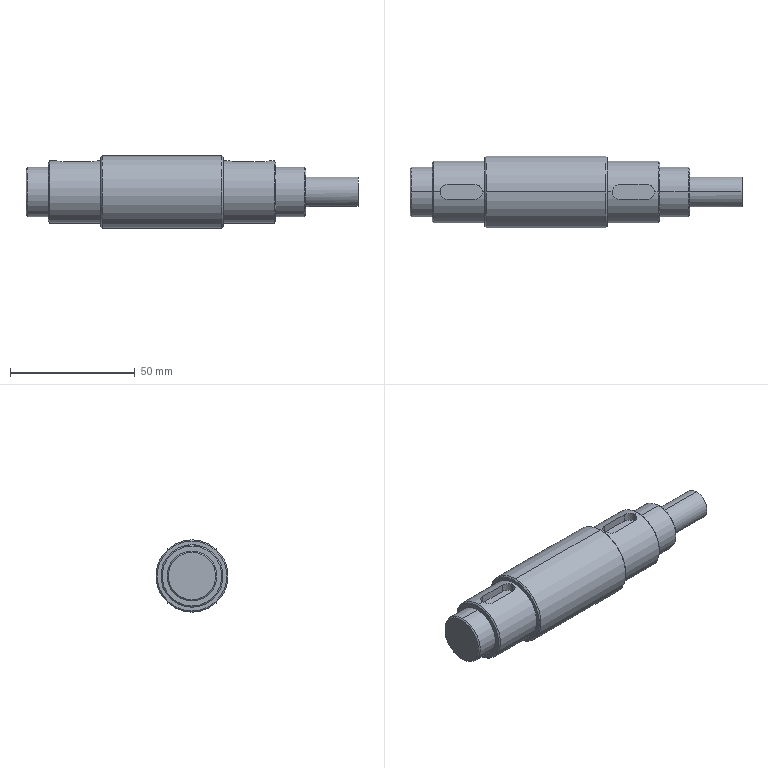Part | NX | features BREP 1 | 1 solid | 52 faces | box 133 x 29 x 29 mm | volume 61010 mm3 | cylinder 22 | plane 16 | cone 14 | commonest cylinder face diameters 6 x6 20 x4 25 x4 3.3 x2 4 x2 12 x2
STEP:
#1=CARTESIAN_POINT('',(-45.5,0.,12.));
#2=VERTEX_POINT('',#1);
#3=CARTESIAN_POINT('',(-45.5,0.,-12.));
#4=VERTEX_POINT('',#3);
#5=CARTESIAN_POINT('',(-45.5,0.,0.));
#6=DIRECTION('',(-1.,0.,0.));
#7=DIRECTION('',(0.,0.,-1.));
#8=AXIS2_PLACEMENT_3D('',#5,#6,#7);
#9=CIRCLE('',#8,12.);
#10=EDGE_CURVE('',#2,#4,#9,.T.);
#11=ORIENTED_EDGE('',*,*,#10,.F.);
#12=CARTESIAN_POINT('',(-45.,0.,12.5));
#13=VERTEX_POINT('',#12);
#14=CARTESIAN_POINT('',(-45.5,0.,12.));
#15=DIRECTION('',(0.7071,0.,0.7071));
#16=VECTOR('',#15,1000.);
#17=LINE('',#14,#16);
#18=EDGE_CURVE('',#2,#13,#17,.T.);
#19=ORIENTED_EDGE('',*,*,#18,.T.);
#20=CARTESIAN_POINT('',(-45.,0.,-12.5));
#21=VERTEX_POINT('',#20);
#22=CARTESIAN_POINT('',(-45.,0.,0.));
#23=DIRECTION('',(1.,0.,0.));
#24=DIRECTION('',(0.,0.,-1.));
#25=AXIS2_PLACEMENT_3D('',#22,#23,#24);
#26=CIRCLE('',#25,12.5);
#27=EDGE_CURVE('',#21,#13,#26,.T.);
#28=ORIENTED_EDGE('',*,*,#27,.F.);
#29=CARTESIAN_POINT('',(-45.5,0.,-12.));
#30=DIRECTION('',(0.7071,0.,-0.7071));
#31=VECTOR('',#30,1000.);
#32=LINE('',#29,#31);
#33=EDGE_CURVE('',#4,#21,#32,.T.);
#34=ORIENTED_EDGE('',*,*,#33,.F.);
#35=EDGE_LOOP('',(#11,#19,#28,#34));
#36=FACE_BOUND('',#35,.T.);
#37=CARTESIAN_POINT('',(-45.5,0.,0.));
#38=DIRECTION('',(1.,0.,0.));
#39=DIRECTION('',(0.,0.,-1.));
#40=AXIS2_PLACEMENT_3D('',#37,#38,#39);
#41=CONICAL_SURFACE('',#40,12.,0.7854);
#42=ADVANCED_FACE('',(#36),#41,.T.);
#43=CARTESIAN_POINT('',(45.5,0.,-12.));
#44=VERTEX_POINT('',#43);
#45=CARTESIAN_POINT('',(45.5,0.,12.));
#46=VERTEX_POINT('',#45);
#47=CARTESIAN_POINT('',(45.5,0.,0.));
#48=DIRECTION('',(1.,0.,0.));
#49=DIRECTION('',(0.,0.,1.));
#50=AXIS2_PLACEMENT_3D('',#47,#48,#49);
#51=CIRCLE('',#50,12.);
#52=EDGE_CURVE('',#44,#46,#51,.T.);
#53=ORIENTED_EDGE('',*,*,#52,.F.);
#54=CARTESIAN_POINT('',(45.,0.,-12.5));
#55=VERTEX_POINT('',#54);
#56=CARTESIAN_POINT('',(45.,0.,-12.5));
#57=DIRECTION('',(-0.7071,0.,-0.7071));
#58=VECTOR('',#57,1000.);
#59=LINE('',#56,#58);
#60=EDGE_CURVE('',#55,#44,#59,.F.);
#61=ORIENTED_EDGE('',*,*,#60,.F.);
#62=CARTESIAN_POINT('',(45.,0.,12.5));
#63=VERTEX_POINT('',#62);
#64=CARTESIAN_POINT('',(45.,0.,0.));
#65=DIRECTION('',(-1.,0.,0.));
#66=DIRECTION('',(0.,0.,1.));
#67=AXIS2_PLACEMENT_3D('',#64,#65,#66);
#68=CIRCLE('',#67,12.5);
#69=EDGE_CURVE('',#63,#55,#68,.T.);
#70=ORIENTED_EDGE('',*,*,#69,.F.);
#71=CARTESIAN_POINT('',(45.,0.,12.5));
#72=DIRECTION('',(-0.7071,0.,0.7071));
#73=VECTOR('',#72,1000.);
#74=LINE('',#71,#73);
#75=EDGE_CURVE('',#63,#46,#74,.F.);
#76=ORIENTED_EDGE('',*,*,#75,.T.);
#77=EDGE_LOOP('',(#53,#61,#70,#76));
#78=FACE_BOUND('',#77,.T.);
#79=CARTESIAN_POINT('',(45.,0.,0.));
#80=DIRECTION('',(-1.,0.,0.));
#81=DIRECTION('',(0.,0.,1.));
#82=AXIS2_PLACEMENT_3D('',#79,#80,#81);
#83=CONICAL_SURFACE('',#82,12.5,0.7854);
#84=ADVANCED_FACE('',(#78),#83,.T.);
#85=CARTESIAN_POINT('',(-24.5,0.,14.));
#86=VERTEX_POINT('',#85);
#87=CARTESIAN_POINT('',(-24.5,0.,-14.));
#88=VERTEX_POINT('',#87);
#89=CARTESIAN_POINT('',(-24.5,0.,0.));
#90=DIRECTION('',(-1.,0.,0.));
#91=DIRECTION('',(0.,0.,-1.));
#92=AXIS2_PLACEMENT_3D('',#89,#90,#91);
#93=CIRCLE('',#92,14.);
#94=EDGE_CURVE('',#86,#88,#93,.T.);
#95=ORIENTED_EDGE('',*,*,#94,.F.);
#96=CARTESIAN_POINT('',(-24.,0.,14.5));
#97=VERTEX_POINT('',#96);
#98=CARTESIAN_POINT('',(-24.5,0.,14.));
#99=DIRECTION('',(0.7071,0.,0.7071));
#100=VECTOR('',#99,1000.);
#101=LINE('',#98,#100);
#102=EDGE_CURVE('',#86,#97,#101,.T.);
#103=ORIENTED_EDGE('',*,*,#102,.T.);
#104=CARTESIAN_POINT('',(-24.,0.,-14.5));
#105=VERTEX_POINT('',#104);
#106=CARTESIAN_POINT('',(-24.,0.,0.));
#107=DIRECTION('',(1.,0.,0.));
#108=DIRECTION('',(0.,0.,-1.));
#109=AXIS2_PLACEMENT_3D('',#106,#107,#108);
#110=CIRCLE('',#109,14.5);
#111=EDGE_CURVE('',#105,#97,#110,.T.);
#112=ORIENTED_EDGE('',*,*,#111,.F.);
#113=CARTESIAN_POINT('',(-24.5,0.,-14.));
#114=DIRECTION('',(0.7071,0.,-0.7071));
#115=VECTOR('',#114,1000.);
#116=LINE('',#113,#115);
#117=EDGE_CURVE('',#88,#105,#116,.T.);
#118=ORIENTED_EDGE('',*,*,#117,.F.);
#119=EDGE_LOOP('',(#95,#103,#112,#118));
#120=FACE_BOUND('',#119,.T.);
#121=CARTESIAN_POINT('',(-24.5,0.,0.));
#122=DIRECTION('',(1.,0.,0.));
#123=DIRECTION('',(0.,0.,-1.));
#124=AXIS2_PLACEMENT_3D('',#121,#122,#123);
#125=CONICAL_SURFACE('',#124,14.,0.7854);
#126=ADVANCED_FACE('',(#120),#125,.T.);
#127=CARTESIAN_POINT('',(24.5,0.,-14.));
#128=VERTEX_POINT('',#127);
#129=CARTESIAN_POINT('',(24.5,0.,14.));
#130=VERTEX_POINT('',#129);
#131=CARTESIAN_POINT('',(24.5,0.,0.));
#132=DIRECTION('',(1.,0.,0.));
#133=DIRECTION('',(0.,0.,1.));
#134=AXIS2_PLACEMENT_3D('',#131,#132,#133);
#135=CIRCLE('',#134,14.);
#136=EDGE_CURVE('',#128,#130,#135,.T.);
#137=ORIENTED_EDGE('',*,*,#136,.F.);
#138=CARTESIAN_POINT('',(24.,0.,-14.5));
#139=VERTEX_POINT('',#138);
#140=CARTESIAN_POINT('',(24.,0.,-14.5));
#141=DIRECTION('',(-0.7071,0.,-0.7071));
#142=VECTOR('',#141,1000.);
#143=LINE('',#140,#142);
#144=EDGE_CURVE('',#139,#128,#143,.F.);
#145=ORIENTED_EDGE('',*,*,#144,.F.);
#146=CARTESIAN_POINT('',(24.,0.,14.5));
#147=VERTEX_POINT('',#146);
#148=CARTESIAN_POINT('',(24.,0.,0.));
#149=DIRECTION('',(-1.,0.,0.));
#150=DIRECTION('',(0.,0.,1.));
#151=AXIS2_PLACEMENT_3D('',#148,#149,#150);
#152=CIRCLE('',#151,14.5);
#153=EDGE_CURVE('',#147,#139,#152,.T.);
#154=ORIENTED_EDGE('',*,*,#153,.F.);
#155=CARTESIAN_POINT('',(24.,0.,14.5));
#156=DIRECTION('',(-0.7071,0.,0.7071));
#157=VECTOR('',#156,1000.);
#158=LINE('',#155,#157);
#159=EDGE_CURVE('',#147,#130,#158,.F.);
#160=ORIENTED_EDGE('',*,*,#159,.T.);
#161=EDGE_LOOP('',(#137,#145,#154,#160));
#162=FACE_BOUND('',#161,.T.);
#163=CARTESIAN_POINT('',(24.,0.,0.));
#164=DIRECTION('',(-1.,0.,0.));
#165=DIRECTION('',(0.,0.,1.));
#166=AXIS2_PLACEMENT_3D('',#163,#164,#165);
#167=CONICAL_SURFACE('',#166,14.5,0.7854);
#168=ADVANCED_FACE('',(#162),#167,.T.);
#169=CARTESIAN_POINT('',(57.5,0.,-9.5));
#170=VERTEX_POINT('',#169);
#171=CARTESIAN_POINT('',(57.5,0.,9.5));
#172=VERTEX_POINT('',#171);
#173=CARTESIAN_POINT('',(57.5,0.,0.));
#174=DIRECTION('',(1.,0.,0.));
#175=DIRECTION('',(0.,0.,1.));
#176=AXIS2_PLACEMENT_3D('',#173,#174,#175);
#177=CIRCLE('',#176,9.5);
#178=EDGE_CURVE('',#170,#172,#177,.T.);
#179=ORIENTED_EDGE('',*,*,#178,.F.);
#180=CARTESIAN_POINT('',(57.,0.,-10.));
#181=VERTEX_POINT('',#180);
#182=CARTESIAN_POINT('',(57.,0.,-10.));
#183=DIRECTION('',(-0.7071,0.,-0.7071));
#184=VECTOR('',#183,1000.);
#185=LINE('',#182,#184);
#186=EDGE_CURVE('',#181,#170,#185,.F.);
#187=ORIENTED_EDGE('',*,*,#186,.F.);
#188=CARTESIAN_POINT('',(57.,0.,10.));
#189=VERTEX_POINT('',#188);
#190=CARTESIAN_POINT('',(57.,0.,0.));
#191=DIRECTION('',(-1.,0.,0.));
#192=DIRECTION('',(0.,0.,1.));
#193=AXIS2_PLACEMENT_3D('',#190,#191,#192);
#194=CIRCLE('',#193,10.);
#195=EDGE_CURVE('',#189,#181,#194,.T.);
#196=ORIENTED_EDGE('',*,*,#195,.F.);
#197=CARTESIAN_POINT('',(57.,0.,10.));
#198=DIRECTION('',(-0.7071,0.,0.7071));
#199=VECTOR('',#198,1000.);
#200=LINE('',#197,#199);
#201=EDGE_CURVE('',#189,#172,#200,.F.);
#202=ORIENTED_EDGE('',*,*,#201,.T.);
#203=EDGE_LOOP('',(#179,#187,#196,#202));
#204=FACE_BOUND('',#203,.T.);
#205=CARTESIAN_POINT('',(57.,0.,0.));
#206=DIRECTION('',(-1.,0.,0.));
#207=DIRECTION('',(0.,0.,1.));
#208=AXIS2_PLACEMENT_3D('',#205,#206,#207);
#209=CONICAL_SURFACE('',#208,10.,0.7854);
#210=ADVANCED_FACE('',(#204),#209,.T.);
#211=CARTESIAN_POINT('',(-54.5,0.,9.5));
#212=VERTEX_POINT('',#211);
#213=CARTESIAN_POINT('',(-54.5,0.,-9.5));
#214=VERTEX_POINT('',#213);
#215=CARTESIAN_POINT('',(-54.5,0.,0.));
#216=DIRECTION('',(-1.,0.,0.));
#217=DIRECTION('',(0.,0.,-1.));
#218=AXIS2_PLACEMENT_3D('',#215,#216,#217);
#219=CIRCLE('',#218,9.5);
#220=EDGE_CURVE('',#212,#214,#219,.T.);
#221=ORIENTED_EDGE('',*,*,#220,.F.);
#222=CARTESIAN_POINT('',(-54.,0.,10.));
#223=VERTEX_POINT('',#222);
#224=CARTESIAN_POINT('',(-54.5,0.,9.5));
#225=DIRECTION('',(0.7071,0.,0.7071));
#226=VECTOR('',#225,1000.);
#227=LINE('',#224,#226);
#228=EDGE_CURVE('',#212,#223,#227,.T.);
#229=ORIENTED_EDGE('',*,*,#228,.T.);
#230=CARTESIAN_POINT('',(-54.,0.,-10.));
#231=VERTEX_POINT('',#230);
#232=CARTESIAN_POINT('',(-54.,0.,0.));
#233=DIRECTION('',(1.,0.,0.));
#234=DIRECTION('',(0.,0.,-1.));
#235=AXIS2_PLACEMENT_3D('',#232,#233,#234);
#236=CIRCLE('',#235,10.);
#237=EDGE_CURVE('',#231,#223,#236,.T.);
#238=ORIENTED_EDGE('',*,*,#237,.F.);
#239=CARTESIAN_POINT('',(-54.5,0.,-9.5));
#240=DIRECTION('',(0.7071,0.,-0.7071));
#241=VECTOR('',#240,1000.);
#242=LINE('',#239,#241);
#243=EDGE_CURVE('',#214,#231,#242,.T.);
#244=ORIENTED_EDGE('',*,*,#243,.F.);
#245=EDGE_LOOP('',(#221,#229,#238,#244));
#246=FACE_BOUND('',#245,.T.);
#247=CARTESIAN_POINT('',(-54.5,0.,0.));
#248=DIRECTION('',(1.,0.,0.));
#249=DIRECTION('',(0.,0.,-1.));
#250=AXIS2_PLACEMENT_3D('',#247,#248,#249);
#251=CONICAL_SURFACE('',#250,9.5,0.7854);
#252=ADVANCED_FACE('',(#246),#251,.T.);
#253=CARTESIAN_POINT('',(67.,0.,1.65));
#254=VERTEX_POINT('',#253);
#255=CARTESIAN_POINT('',(67.,0.,-1.65));
#256=VERTEX_POINT('',#255);
#257=CARTESIAN_POINT('',(67.,0.,0.));
#258=DIRECTION('',(1.,0.,0.));
#259=DIRECTION('',(0.,0.,-1.));
#260=AXIS2_PLACEMENT_3D('',#257,#258,#259);
#261=CIRCLE('',#260,1.65);
#262=EDGE_CURVE('',#254,#256,#261,.T.);
#263=ORIENTED_EDGE('',*,*,#262,.F.);
#264=CARTESIAN_POINT('',(78.5,0.,1.65));
#265=VERTEX_POINT('',#264);
#266=CARTESIAN_POINT('',(78.5,0.,1.65));
#267=DIRECTION('',(1.,0.,0.));
#268=VECTOR('',#267,1000.);
#269=LINE('',#266,#268);
#270=EDGE_CURVE('',#254,#265,#269,.T.);
#271=ORIENTED_EDGE('',*,*,#270,.T.);
#272=CARTESIAN_POINT('',(78.5,0.,-1.65));
#273=VERTEX_POINT('',#272);
#274=CARTESIAN_POINT('',(78.5,0.,0.));
#275=DIRECTION('',(1.,0.,0.));
#276=DIRECTION('',(0.,0.,-1.));
#277=AXIS2_PLACEMENT_3D('',#274,#275,#276);
#278=CIRCLE('',#277,1.65);
#279=EDGE_CURVE('',#265,#273,#278,.T.);
#280=ORIENTED_EDGE('',*,*,#279,.T.);
#281=CARTESIAN_POINT('',(78.5,0.,-1.65));
#282=DIRECTION('',(1.,0.,0.));
#283=VECTOR('',#282,1000.);
#284=LINE('',#281,#283);
#285=EDGE_CURVE('',#256,#273,#284,.T.);
#286=ORIENTED_EDGE('',*,*,#285,.F.);
#287=EDGE_LOOP('',(#263,#271,#280,#286));
#288=FACE_BOUND('',#287,.T.);
#289=CARTESIAN_POINT('',(78.5,0.,0.));
#290=DIRECTION('',(1.,0.,0.));
#291=DIRECTION('',(0.,0.,-1.));
#292=AXIS2_PLACEMENT_3D('',#289,#290,#291);
#293=CYLINDRICAL_SURFACE('',#292,1.65);
#294=ADVANCED_FACE('',(#288),#293,.F.);
#295=CARTESIAN_POINT('',(66.009,0.,0.));
#296=VERTEX_POINT('',#295);
#297=CARTESIAN_POINT('',(67.,0.,-1.65));
#298=DIRECTION('',(0.515,0.,-0.8572));
#299=VECTOR('',#298,1000.);
#300=LINE('',#297,#299);
#301=EDGE_CURVE('',#296,#256,#300,.T.);
#302=ORIENTED_EDGE('',*,*,#301,.F.);
#303=CARTESIAN_POINT('',(67.,0.,1.65));
#304=DIRECTION('',(0.515,0.,0.8572));
#305=VECTOR('',#304,1000.);
#306=LINE('',#303,#305);
#307=EDGE_CURVE('',#296,#254,#306,.T.);
#308=ORIENTED_EDGE('',*,*,#307,.T.);
#309=ORIENTED_EDGE('',*,*,#262,.T.);
#310=EDGE_LOOP('',(#302,#308,#309));
#311=FACE_BOUND('',#310,.T.);
#312=CARTESIAN_POINT('',(67.,0.,0.));
#313=DIRECTION('',(1.,0.,0.));
#314=DIRECTION('',(0.,0.,-1.));
#315=AXIS2_PLACEMENT_3D('',#312,#313,#314);
#316=CONICAL_SURFACE('',#315,1.65,1.03);
#317=ADVANCED_FACE('',(#311),#316,.F.);
#318=CARTESIAN_POINT('',(-25.5,0.,9.));
#319=VERTEX_POINT('',#318);
#320=CARTESIAN_POINT('',(-28.5,3.,9.));
#321=VERTEX_POINT('',#320);
#322=CARTESIAN_POINT('',(-28.5,0.,9.));
#323=DIRECTION('',(0.,0.,1.));
#324=DIRECTION('',(1.,0.,0.));
#325=AXIS2_PLACEMENT_3D('',#322,#323,#324);
#326=CIRCLE('',#325,3.);
#327=EDGE_CURVE('',#319,#321,#326,.T.);
#328=ORIENTED_EDGE('',*,*,#327,.F.);
#329=CARTESIAN_POINT('',(-25.5,0.,12.5));
#330=VERTEX_POINT('',#329);
#331=CARTESIAN_POINT('',(-25.5,0.,9.));
#332=DIRECTION('',(0.,0.,1.));
#333=VECTOR('',#332,1000.);
#334=LINE('',#331,#333);
#335=EDGE_CURVE('',#319,#330,#334,.T.);
#336=ORIENTED_EDGE('',*,*,#335,.T.);
#337=CARTESIAN_POINT('',(-28.5,3.,12.135));
#338=VERTEX_POINT('',#337);
#339=CARTESIAN_POINT('',(-25.5,0.,12.5));
#340=CARTESIAN_POINT('',(-25.5,0.3726,12.5));
#341=CARTESIAN_POINT('',(-25.616,0.9196,12.472));
#342=CARTESIAN_POINT('',(-25.836,1.392,12.423));
#343=CARTESIAN_POINT('',(-26.017,1.691,12.386));
#344=CARTESIAN_POINT('',(-26.135,1.851,12.362));
#345=CARTESIAN_POINT('',(-26.368,2.125,12.319));
#346=CARTESIAN_POINT('',(-26.658,2.372,12.273));
#347=CARTESIAN_POINT('',(-26.805,2.48,12.252));
#348=CARTESIAN_POINT('',(-27.11,2.665,12.213));
#349=CARTESIAN_POINT('',(-27.574,2.88,12.164));
#350=CARTESIAN_POINT('',(-28.128,3.,12.135));
#351=CARTESIAN_POINT('',(-28.5,3.,12.135));
#352=B_SPLINE_CURVE_WITH_KNOTS('',3,(#339,#340,#341,#342,#343,#344,#345,#346,#347,#348,#349,#350,#351),.UNSPECIFIED.,.F.,.F.,(4,1,1,1,1,1,1,1,1,1,4),(0.,0.25,0.3125,0.375,0.4375,0.5,0.5625,0.625,0.6875,0.75,1.),.UNSPECIFIED.);
#353=EDGE_CURVE('',#338,#330,#352,.F.);
#354=ORIENTED_EDGE('',*,*,#353,.F.);
#355=CARTESIAN_POINT('',(-28.5,3.,9.));
#356=DIRECTION('',(0.,0.,1.));
#357=VECTOR('',#356,1000.);
#358=LINE('',#355,#357);
#359=EDGE_CURVE('',#321,#338,#358,.T.);
#360=ORIENTED_EDGE('',*,*,#359,.F.);
#361=EDGE_LOOP('',(#328,#336,#354,#360));
#362=FACE_BOUND('',#361,.T.);
#363=CARTESIAN_POINT('',(-28.5,0.,9.));
#364=DIRECTION('',(0.,0.,1.));
#365=DIRECTION('',(1.,0.,0.));
#366=AXIS2_PLACEMENT_3D('',#363,#364,#365);
#367=CYLINDRICAL_SURFACE('',#366,3.);
#368=ADVANCED_FACE('',(#362),#367,.F.);
#369=CARTESIAN_POINT('',(60.5,2.,-5.657));
#370=VERTEX_POINT('',#369);
#371=CARTESIAN_POINT('',(58.5,0.,-6.));
#372=VERTEX_POINT('',#371);
#373=CARTESIAN_POINT('',(60.5,2.,-5.657));
#374=CARTESIAN_POINT('',(59.437,1.999,-5.657));
#375=CARTESIAN_POINT('',(58.5,1.066,-6.));
#376=CARTESIAN_POINT('',(58.5,0.,-6.));
#377=B_SPLINE_CURVE_WITH_KNOTS('',3,(#373,#374,#375,#376),.UNSPECIFIED.,.F.,.F.,(4,4),(0.,1.),.UNSPECIFIED.);
#378=EDGE_CURVE('',#370,#372,#377,.T.);
#379=ORIENTED_EDGE('',*,*,#378,.T.);
#380=CARTESIAN_POINT('',(57.5,0.,-6.));
#381=VERTEX_POINT('',#380);
#382=CARTESIAN_POINT('',(78.5,0.,-6.));
#383=DIRECTION('',(-1.,0.,0.));
#384=VECTOR('',#383,1000.);
#385=LINE('',#382,#384);
#386=EDGE_CURVE('',#381,#372,#385,.F.);
#387=ORIENTED_EDGE('',*,*,#386,.F.);
#388=CARTESIAN_POINT('',(57.5,0.,6.));
#389=VERTEX_POINT('',#388);
#390=CARTESIAN_POINT('',(57.5,0.,0.));
#391=DIRECTION('',(1.,0.,0.));
#392=DIRECTION('',(0.,0.,1.));
#393=AXIS2_PLACEMENT_3D('',#390,#391,#392);
#394=CIRCLE('',#393,6.);
#395=EDGE_CURVE('',#381,#389,#394,.T.);
#396=ORIENTED_EDGE('',*,*,#395,.T.);
#397=CARTESIAN_POINT('',(78.5,0.,6.));
#398=VERTEX_POINT('',#397);
#399=CARTESIAN_POINT('',(78.5,0.,6.));
#400=DIRECTION('',(-1.,0.,0.));
#401=VECTOR('',#400,1000.);
#402=LINE('',#399,#401);
#403=EDGE_CURVE('',#389,#398,#402,.F.);
#404=ORIENTED_EDGE('',*,*,#403,.T.);
#405=CARTESIAN_POINT('',(78.5,2.,-5.657));
#406=VERTEX_POINT('',#405);
#407=CARTESIAN_POINT('',(78.5,0.,0.));
#408=DIRECTION('',(1.,0.,0.));
#409=DIRECTION('',(0.,0.,-1.));
#410=AXIS2_PLACEMENT_3D('',#407,#408,#409);
#411=CIRCLE('',#410,6.);
#412=EDGE_CURVE('',#406,#398,#411,.T.);
#413=ORIENTED_EDGE('',*,*,#412,.F.);
#414=CARTESIAN_POINT('',(78.5,2.,-5.657));
#415=DIRECTION('',(-1.,0.,0.));
#416=VECTOR('',#415,1000.);
#417=LINE('',#414,#416);
#418=EDGE_CURVE('',#406,#370,#417,.T.);
#419=ORIENTED_EDGE('',*,*,#418,.T.);
#420=EDGE_LOOP('',(#379,#387,#396,#404,#413,#419));
#421=FACE_BOUND('',#420,.T.);
#422=CARTESIAN_POINT('',(78.5,0.,0.));
#423=DIRECTION('',(-1.,0.,0.));
#424=DIRECTION('',(0.,0.,1.));
#425=AXIS2_PLACEMENT_3D('',#422,#423,#424);
#426=CYLINDRICAL_SURFACE('',#425,6.);
#427=ADVANCED_FACE('',(#421),#426,.T.);
#428=CARTESIAN_POINT('',(43.5,0.,9.));
#429=VERTEX_POINT('',#428);
#430=CARTESIAN_POINT('',(40.5,3.,9.));
#431=VERTEX_POINT('',#430);
#432=CARTESIAN_POINT('',(40.5,0.,9.));
#433=DIRECTION('',(0.,0.,1.));
#434=DIRECTION('',(1.,0.,0.));
#435=AXIS2_PLACEMENT_3D('',#432,#433,#434);
#436=CIRCLE('',#435,3.);
#437=EDGE_CURVE('',#429,#431,#436,.T.);
#438=ORIENTED_EDGE('',*,*,#437,.F.);
#439=CARTESIAN_POINT('',(43.5,0.,12.5));
#440=VERTEX_POINT('',#439);
#441=CARTESIAN_POINT('',(43.5,0.,9.));
#442=DIRECTION('',(0.,0.,1.));
#443=VECTOR('',#442,1000.);
#444=LINE('',#441,#443);
#445=EDGE_CURVE('',#429,#440,#444,.T.);
#446=ORIENTED_EDGE('',*,*,#445,.T.);
#447=CARTESIAN_POINT('',(40.5,3.,12.135));
#448=VERTEX_POINT('',#447);
#449=CARTESIAN_POINT('',(43.5,0.,12.5));
#450=CARTESIAN_POINT('',(43.5,0.3726,12.5));
#451=CARTESIAN_POINT('',(43.384,0.9196,12.472));
#452=CARTESIAN_POINT('',(43.164,1.392,12.423));
#453=CARTESIAN_POINT('',(42.983,1.691,12.386));
#454=CARTESIAN_POINT('',(42.865,1.851,12.362));
#455=CARTESIAN_POINT('',(42.632,2.125,12.319));
#456=CARTESIAN_POINT('',(42.342,2.372,12.273));
#457=CARTESIAN_POINT('',(42.195,2.48,12.252));
#458=CARTESIAN_POINT('',(41.89,2.665,12.213));
#459=CARTESIAN_POINT('',(41.426,2.88,12.164));
#460=CARTESIAN_POINT('',(40.872,3.,12.135));
#461=CARTESIAN_POINT('',(40.5,3.,12.135));
#462=B_SPLINE_CURVE_WITH_KNOTS('',3,(#449,#450,#451,#452,#453,#454,#455,#456,#457,#458,#459,#460,#461),.UNSPECIFIED.,.F.,.F.,(4,1,1,1,1,1,1,1,1,1,4),(0.,0.25,0.3125,0.375,0.4375,0.5,0.5625,0.625,0.6875,0.75,1.),.UNSPECIFIED.);
#463=EDGE_CURVE('',#448,#440,#462,.F.);
#464=ORIENTED_EDGE('',*,*,#463,.F.);
#465=CARTESIAN_POINT('',(40.5,3.,9.));
#466=DIRECTION('',(0.,0.,1.));
#467=VECTOR('',#466,1000.);
#468=LINE('',#465,#467);
#469=EDGE_CURVE('',#431,#448,#468,.T.);
#470=ORIENTED_EDGE('',*,*,#469,.F.);
#471=EDGE_LOOP('',(#438,#446,#464,#470));
#472=FACE_BOUND('',#471,.T.);
#473=CARTESIAN_POINT('',(40.5,0.,9.));
#474=DIRECTION('',(0.,0.,1.));
#475=DIRECTION('',(1.,0.,0.));
#476=AXIS2_PLACEMENT_3D('',#473,#474,#475);
#477=CYLINDRICAL_SURFACE('',#476,3.);
#478=ADVANCED_FACE('',(#472),#477,.F.);
#479=ORIENTED_EDGE('',*,*,#195,.T.);
#480=CARTESIAN_POINT('',(45.5,0.,-10.));
#481=VERTEX_POINT('',#480);
#482=CARTESIAN_POINT('',(-54.5,0.,-10.));
#483=DIRECTION('',(-1.,0.,0.));
#484=VECTOR('',#483,1000.);
#485=LINE('',#482,#484);
#486=EDGE_CURVE('',#481,#181,#485,.F.);
#487=ORIENTED_EDGE('',*,*,#486,.F.);
#488=CARTESIAN_POINT('',(45.5,0.,10.));
#489=VERTEX_POINT('',#488);
#490=CARTESIAN_POINT('',(45.5,0.,0.));
#491=DIRECTION('',(-1.,0.,0.));
#492=DIRECTION('',(0.,0.,1.));
#493=AXIS2_PLACEMENT_3D('',#490,#491,#492);
#494=CIRCLE('',#493,10.);
#495=EDGE_CURVE('',#489,#481,#494,.T.);
#496=ORIENTED_EDGE('',*,*,#495,.F.);
#497=CARTESIAN_POINT('',(-54.5,0.,10.));
#498=DIRECTION('',(-1.,0.,0.));
#499=VECTOR('',#498,1000.);
#500=LINE('',#497,#499);
#501=EDGE_CURVE('',#489,#189,#500,.F.);
#502=ORIENTED_EDGE('',*,*,#501,.T.);
#503=EDGE_LOOP('',(#479,#487,#496,#502));
#504=FACE_BOUND('',#503,.T.);
#505=CARTESIAN_POINT('',(-54.5,0.,0.));
#506=DIRECTION('',(-1.,0.,0.));
#507=DIRECTION('',(0.,0.,1.));
#508=AXIS2_PLACEMENT_3D('',#505,#506,#507);
#509=CYLINDRICAL_SURFACE('',#508,10.);
#510=ADVANCED_FACE('',(#504),#509,.T.);
#511=ORIENTED_EDGE('',*,*,#69,.T.);
#512=CARTESIAN_POINT('',(24.5,0.,-12.5));
#513=VERTEX_POINT('',#512);
#514=CARTESIAN_POINT('',(-54.5,0.,-12.5));
#515=DIRECTION('',(-1.,0.,0.));
#516=VECTOR('',#515,1000.);
#517=LINE('',#514,#516);
#518=EDGE_CURVE('',#513,#55,#517,.F.);
#519=ORIENTED_EDGE('',*,*,#518,.F.);
#520=CARTESIAN_POINT('',(24.5,0.,12.5));
#521=VERTEX_POINT('',#520);
#522=CARTESIAN_POINT('',(24.5,0.,0.));
#523=DIRECTION('',(-1.,0.,0.));
#524=DIRECTION('',(0.,0.,1.));
#525=AXIS2_PLACEMENT_3D('',#522,#523,#524);
#526=CIRCLE('',#525,12.5);
#527=EDGE_CURVE('',#521,#513,#526,.T.);
#528=ORIENTED_EDGE('',*,*,#527,.F.);
#529=CARTESIAN_POINT('',(26.5,0.,12.5));
#530=VERTEX_POINT('',#529);
#531=CARTESIAN_POINT('',(-54.5,0.,12.5));
#532=DIRECTION('',(-1.,0.,0.));
#533=VECTOR('',#532,1000.);
#534=LINE('',#531,#533);
#535=EDGE_CURVE('',#530,#521,#534,.T.);
#536=ORIENTED_EDGE('',*,*,#535,.F.);
#537=CARTESIAN_POINT('',(29.5,3.,12.135));
#538=VERTEX_POINT('',#537);
#539=CARTESIAN_POINT('',(26.5,0.,12.5));
#540=CARTESIAN_POINT('',(26.5,0.7917,12.5));
#541=CARTESIAN_POINT('',(27.156,2.347,12.32));
#542=CARTESIAN_POINT('',(28.703,3.,12.135));
#543=CARTESIAN_POINT('',(29.5,3.,12.135));
#544=B_SPLINE_CURVE_WITH_KNOTS('',3,(#539,#540,#541,#542,#543),.UNSPECIFIED.,.F.,.F.,(4,1,4),(0.,0.5,1.),.UNSPECIFIED.);
#545=EDGE_CURVE('',#530,#538,#544,.T.);
#546=ORIENTED_EDGE('',*,*,#545,.T.);
#547=CARTESIAN_POINT('',(-54.5,3.,12.135));
#548=DIRECTION('',(1.,0.,0.));
#549=VECTOR('',#548,1000.);
#550=LINE('',#547,#549);
#551=EDGE_CURVE('',#538,#448,#550,.T.);
#552=ORIENTED_EDGE('',*,*,#551,.T.);
#553=ORIENTED_EDGE('',*,*,#463,.T.);
#554=CARTESIAN_POINT('',(-54.5,0.,12.5));
#555=DIRECTION('',(-1.,0.,0.));
#556=VECTOR('',#555,1000.);
#557=LINE('',#554,#556);
#558=EDGE_CURVE('',#440,#63,#557,.F.);
#559=ORIENTED_EDGE('',*,*,#558,.T.);
#560=EDGE_LOOP('',(#511,#519,#528,#536,#546,#552,#553,#559));
#561=FACE_BOUND('',#560,.T.);
#562=CARTESIAN_POINT('',(-54.5,0.,0.));
#563=DIRECTION('',(-1.,0.,0.));
#564=DIRECTION('',(0.,0.,1.));
#565=AXIS2_PLACEMENT_3D('',#562,#563,#564);
#566=CYLINDRICAL_SURFACE('',#565,12.5);
#567=ADVANCED_FACE('',(#561),#566,.T.);
#568=ORIENTED_EDGE('',*,*,#153,.T.);
#569=CARTESIAN_POINT('',(-54.5,0.,-14.5));
#570=DIRECTION('',(-1.,0.,0.));
#571=VECTOR('',#570,1000.);
#572=LINE('',#569,#571);
#573=EDGE_CURVE('',#105,#139,#572,.F.);
#574=ORIENTED_EDGE('',*,*,#573,.F.);
#575=ORIENTED_EDGE('',*,*,#111,.T.);
#576=CARTESIAN_POINT('',(-54.5,0.,14.5));
#577=DIRECTION('',(-1.,0.,0.));
#578=VECTOR('',#577,1000.);
#579=LINE('',#576,#578);
#580=EDGE_CURVE('',#97,#147,#579,.F.);
#581=ORIENTED_EDGE('',*,*,#580,.T.);
#582=EDGE_LOOP('',(#568,#574,#575,#581));
#583=FACE_BOUND('',#582,.T.);
#584=CARTESIAN_POINT('',(-54.5,0.,0.));
#585=DIRECTION('',(-1.,0.,0.));
#586=DIRECTION('',(0.,0.,1.));
#587=AXIS2_PLACEMENT_3D('',#584,#585,#586);
#588=CYLINDRICAL_SURFACE('',#587,14.5);
#589=ADVANCED_FACE('',(#583),#588,.T.);
#590=CARTESIAN_POINT('',(-24.5,0.,12.5));
#591=VERTEX_POINT('',#590);
#592=CARTESIAN_POINT('',(-24.5,0.,-12.5));
#593=VERTEX_POINT('',#592);
#594=CARTESIAN_POINT('',(-24.5,0.,0.));
#595=DIRECTION('',(-1.,0.,0.));
#596=DIRECTION('',(0.,0.,1.));
#597=AXIS2_PLACEMENT_3D('',#594,#595,#596);
#598=CIRCLE('',#597,12.5);
#599=EDGE_CURVE('',#591,#593,#598,.T.);
#600=ORIENTED_EDGE('',*,*,#599,.T.);
#601=CARTESIAN_POINT('',(-54.5,0.,-12.5));
#602=DIRECTION('',(-1.,0.,0.));
#603=VECTOR('',#602,1000.);
#604=LINE('',#601,#603);
#605=EDGE_CURVE('',#21,#593,#604,.F.);
#606=ORIENTED_EDGE('',*,*,#605,.F.);
#607=ORIENTED_EDGE('',*,*,#27,.T.);
#608=CARTESIAN_POINT('',(-42.5,0.,12.5));
#609=VERTEX_POINT('',#608);
#610=CARTESIAN_POINT('',(-54.5,0.,12.5));
#611=DIRECTION('',(-1.,0.,0.));
#612=VECTOR('',#611,1000.);
#613=LINE('',#610,#612);
#614=EDGE_CURVE('',#609,#13,#613,.T.);
#615=ORIENTED_EDGE('',*,*,#614,.F.);
#616=CARTESIAN_POINT('',(-39.5,3.,12.135));
#617=VERTEX_POINT('',#616);
#618=CARTESIAN_POINT('',(-42.5,0.,12.5));
#619=CARTESIAN_POINT('',(-42.5,0.7917,12.5));
#620=CARTESIAN_POINT('',(-41.844,2.347,12.32));
#621=CARTESIAN_POINT('',(-40.297,3.,12.135));
#622=CARTESIAN_POINT('',(-39.5,3.,12.135));
#623=B_SPLINE_CURVE_WITH_KNOTS('',3,(#618,#619,#620,#621,#622),.UNSPECIFIED.,.F.,.F.,(4,1,4),(0.,0.5,1.),.UNSPECIFIED.);
#624=EDGE_CURVE('',#609,#617,#623,.T.);
#625=ORIENTED_EDGE('',*,*,#624,.T.);
#626=CARTESIAN_POINT('',(-54.5,3.,12.135));
#627=DIRECTION('',(1.,0.,0.));
#628=VECTOR('',#627,1000.);
#629=LINE('',#626,#628);
#630=EDGE_CURVE('',#617,#338,#629,.T.);
#631=ORIENTED_EDGE('',*,*,#630,.T.);
#632=ORIENTED_EDGE('',*,*,#353,.T.);
#633=CARTESIAN_POINT('',(-54.5,0.,12.5));
#634=DIRECTION('',(-1.,0.,0.));
#635=VECTOR('',#634,1000.);
#636=LINE('',#633,#635);
#637=EDGE_CURVE('',#330,#591,#636,.F.);
#638=ORIENTED_EDGE('',*,*,#637,.T.);
#639=EDGE_LOOP('',(#600,#606,#607,#615,#625,#631,#632,#638));
#640=FACE_BOUND('',#639,.T.);
#641=CARTESIAN_POINT('',(-54.5,0.,0.));
#642=DIRECTION('',(-1.,0.,0.));
#643=DIRECTION('',(0.,0.,1.));
#644=AXIS2_PLACEMENT_3D('',#641,#642,#643);
#645=CYLINDRICAL_SURFACE('',#644,12.5);
#646=ADVANCED_FACE('',(#640),#645,.T.);
#647=CARTESIAN_POINT('',(-45.5,0.,10.));
#648=VERTEX_POINT('',#647);
#649=CARTESIAN_POINT('',(-45.5,0.,-10.));
#650=VERTEX_POINT('',#649);
#651=CARTESIAN_POINT('',(-45.5,0.,0.));
#652=DIRECTION('',(-1.,0.,0.));
#653=DIRECTION('',(0.,0.,1.));
#654=AXIS2_PLACEMENT_3D('',#651,#652,#653);
#655=CIRCLE('',#654,10.);
#656=EDGE_CURVE('',#648,#650,#655,.T.);
#657=ORIENTED_EDGE('',*,*,#656,.T.);
#658=CARTESIAN_POINT('',(-54.5,0.,-10.));
#659=DIRECTION('',(-1.,0.,0.));
#660=VECTOR('',#659,1000.);
#661=LINE('',#658,#660);
#662=EDGE_CURVE('',#231,#650,#661,.F.);
#663=ORIENTED_EDGE('',*,*,#662,.F.);
#664=ORIENTED_EDGE('',*,*,#237,.T.);
#665=CARTESIAN_POINT('',(-54.5,0.,10.));
#666=DIRECTION('',(-1.,0.,0.));
#667=VECTOR('',#666,1000.);
#668=LINE('',#665,#667);
#669=EDGE_CURVE('',#223,#648,#668,.F.);
#670=ORIENTED_EDGE('',*,*,#669,.T.);
#671=EDGE_LOOP('',(#657,#663,#664,#670));
#672=FACE_BOUND('',#671,.T.);
#673=CARTESIAN_POINT('',(-54.5,0.,0.));
#674=DIRECTION('',(-1.,0.,0.));
#675=DIRECTION('',(0.,0.,1.));
#676=AXIS2_PLACEMENT_3D('',#673,#674,#675);
#677=CYLINDRICAL_SURFACE('',#676,10.);
#678=ADVANCED_FACE('',(#672),#677,.T.);
#679=CARTESIAN_POINT('',(57.5,0.,0.));
#680=DIRECTION('',(1.,0.,0.));
#681=DIRECTION('',(0.,0.,1.));
#682=AXIS2_PLACEMENT_3D('',#679,#680,#681);
#683=CIRCLE('',#682,9.5);
#684=EDGE_CURVE('',#172,#170,#683,.T.);
#685=ORIENTED_EDGE('',*,*,#684,.T.);
#686=ORIENTED_EDGE('',*,*,#178,.T.);
#687=EDGE_LOOP('',(#685,#686));
#688=FACE_BOUND('',#687,.T.);
#689=CARTESIAN_POINT('',(57.5,0.,0.));
#690=DIRECTION('',(1.,0.,0.));
#691=DIRECTION('',(0.,0.,1.));
#692=AXIS2_PLACEMENT_3D('',#689,#690,#691);
#693=CIRCLE('',#692,6.);
#694=EDGE_CURVE('',#389,#381,#693,.T.);
#695=ORIENTED_EDGE('',*,*,#694,.F.);
#696=ORIENTED_EDGE('',*,*,#395,.F.);
#697=EDGE_LOOP('',(#695,#696));
#698=FACE_BOUND('',#697,.T.);
#699=CARTESIAN_POINT('',(57.5,0.,0.));
#700=DIRECTION('',(-1.,0.,0.));
#701=DIRECTION('',(0.,0.,1.));
#702=AXIS2_PLACEMENT_3D('',#699,#700,#701);
#703=PLANE('',#702);
#704=ADVANCED_FACE('',(#688,#698),#703,.F.);
#705=CARTESIAN_POINT('',(-54.5,0.,0.));
#706=DIRECTION('',(-1.,0.,0.));
#707=DIRECTION('',(0.,0.,-1.));
#708=AXIS2_PLACEMENT_3D('',#705,#706,#707);
#709=CIRCLE('',#708,9.5);
#710=EDGE_CURVE('',#214,#212,#709,.T.);
#711=ORIENTED_EDGE('',*,*,#710,.T.);
#712=ORIENTED_EDGE('',*,*,#220,.T.);
#713=EDGE_LOOP('',(#711,#712));
#714=FACE_BOUND('',#713,.T.);
#715=CARTESIAN_POINT('',(-54.5,0.,0.));
#716=DIRECTION('',(1.,0.,0.));
#717=DIRECTION('',(0.,1.,0.));
#718=AXIS2_PLACEMENT_3D('',#715,#716,#717);
#719=PLANE('',#718);
#720=ADVANCED_FACE('',(#714),#719,.F.);
#721=ORIENTED_EDGE('',*,*,#662,.T.);
#722=CARTESIAN_POINT('',(-45.5,0.,0.));
#723=DIRECTION('',(-1.,0.,0.));
#724=DIRECTION('',(0.,0.,1.));
#725=AXIS2_PLACEMENT_3D('',#722,#723,#724);
#726=CIRCLE('',#725,10.);
#727=EDGE_CURVE('',#650,#648,#726,.T.);
#728=ORIENTED_EDGE('',*,*,#727,.T.);
#729=ORIENTED_EDGE('',*,*,#669,.F.);
#730=CARTESIAN_POINT('',(-54.,0.,0.));
#731=DIRECTION('',(1.,0.,0.));
#732=DIRECTION('',(0.,0.,-1.));
#733=AXIS2_PLACEMENT_3D('',#730,#731,#732);
#734=CIRCLE('',#733,10.);
#735=EDGE_CURVE('',#223,#231,#734,.T.);
#736=ORIENTED_EDGE('',*,*,#735,.T.);
#737=EDGE_LOOP('',(#721,#728,#729,#736));
#738=FACE_BOUND('',#737,.T.);
#739=CARTESIAN_POINT('',(-54.5,0.,0.));
#740=DIRECTION('',(-1.,0.,0.));
#741=DIRECTION('',(0.,0.,1.));
#742=AXIS2_PLACEMENT_3D('',#739,#740,#741);
#743=CYLINDRICAL_SURFACE('',#742,10.);
#744=ADVANCED_FACE('',(#738),#743,.T.);
#745=CARTESIAN_POINT('',(-45.5,0.,0.));
#746=DIRECTION('',(-1.,0.,0.));
#747=DIRECTION('',(0.,0.,-1.));
#748=AXIS2_PLACEMENT_3D('',#745,#746,#747);
#749=CIRCLE('',#748,12.);
#750=EDGE_CURVE('',#4,#2,#749,.T.);
#751=ORIENTED_EDGE('',*,*,#750,.T.);
#752=ORIENTED_EDGE('',*,*,#10,.T.);
#753=EDGE_LOOP('',(#751,#752));
#754=FACE_BOUND('',#753,.T.);
#755=ORIENTED_EDGE('',*,*,#656,.F.);
#756=ORIENTED_EDGE('',*,*,#727,.F.);
#757=EDGE_LOOP('',(#755,#756));
#758=FACE_BOUND('',#757,.T.);
#759=CARTESIAN_POINT('',(-45.5,10.,0.));
#760=DIRECTION('',(1.,0.,0.));
#761=DIRECTION('',(0.,1.,0.));
#762=AXIS2_PLACEMENT_3D('',#759,#760,#761);
#763=PLANE('',#762);
#764=ADVANCED_FACE('',(#754,#758),#763,.F.);
#765=ORIENTED_EDGE('',*,*,#605,.T.);
#766=CARTESIAN_POINT('',(-24.5,0.,0.));
#767=DIRECTION('',(-1.,0.,0.));
#768=DIRECTION('',(0.,0.,1.));
#769=AXIS2_PLACEMENT_3D('',#766,#767,#768);
#770=CIRCLE('',#769,12.5);
#771=EDGE_CURVE('',#593,#591,#770,.T.);
#772=ORIENTED_EDGE('',*,*,#771,.T.);
#773=ORIENTED_EDGE('',*,*,#637,.F.);
#774=CARTESIAN_POINT('',(-28.5,-3.,12.135));
#775=VERTEX_POINT('',#774);
#776=CARTESIAN_POINT('',(-25.5,0.,12.5));
#777=CARTESIAN_POINT('',(-25.5,-0.7917,12.5));
#778=CARTESIAN_POINT('',(-26.156,-2.347,12.32));
#779=CARTESIAN_POINT('',(-27.703,-3.,12.135));
#780=CARTESIAN_POINT('',(-28.5,-3.,12.135));
#781=B_SPLINE_CURVE_WITH_KNOTS('',3,(#776,#777,#778,#779,#780),.UNSPECIFIED.,.F.,.F.,(4,1,4),(0.,0.5,1.),.UNSPECIFIED.);
#782=EDGE_CURVE('',#330,#775,#781,.T.);
#783=ORIENTED_EDGE('',*,*,#782,.T.);
#784=CARTESIAN_POINT('',(-39.5,-3.,12.135));
#785=VERTEX_POINT('',#784);
#786=CARTESIAN_POINT('',(-54.5,-3.,12.135));
#787=DIRECTION('',(-1.,0.,0.));
#788=VECTOR('',#787,1000.);
#789=LINE('',#786,#788);
#790=EDGE_CURVE('',#775,#785,#789,.T.);
#791=ORIENTED_EDGE('',*,*,#790,.T.);
#792=CARTESIAN_POINT('',(-39.5,-3.,12.135));
#793=CARTESIAN_POINT('',(-40.291,-3.,12.135));
#794=CARTESIAN_POINT('',(-41.849,-2.347,12.32));
#795=CARTESIAN_POINT('',(-42.5,-0.7885,12.5));
#796=CARTESIAN_POINT('',(-42.5,0.,12.5));
#797=B_SPLINE_CURVE_WITH_KNOTS('',3,(#792,#793,#794,#795,#796),.UNSPECIFIED.,.F.,.F.,(4,1,4),(0.,0.5,1.),.UNSPECIFIED.);
#798=EDGE_CURVE('',#785,#609,#797,.T.);
#799=ORIENTED_EDGE('',*,*,#798,.T.);
#800=ORIENTED_EDGE('',*,*,#614,.T.);
#801=CARTESIAN_POINT('',(-45.,0.,0.));
#802=DIRECTION('',(1.,0.,0.));
#803=DIRECTION('',(0.,0.,-1.));
#804=AXIS2_PLACEMENT_3D('',#801,#802,#803);
#805=CIRCLE('',#804,12.5);
#806=EDGE_CURVE('',#13,#21,#805,.T.);
#807=ORIENTED_EDGE('',*,*,#806,.T.);
#808=EDGE_LOOP('',(#765,#772,#773,#783,#791,#799,#800,#807));
#809=FACE_BOUND('',#808,.T.);
#810=CARTESIAN_POINT('',(-54.5,0.,0.));
#811=DIRECTION('',(-1.,0.,0.));
#812=DIRECTION('',(0.,0.,1.));
#813=AXIS2_PLACEMENT_3D('',#810,#811,#812);
#814=CYLINDRICAL_SURFACE('',#813,12.5);
#815=ADVANCED_FACE('',(#809),#814,.T.);
#816=CARTESIAN_POINT('',(-24.5,0.,0.));
#817=DIRECTION('',(-1.,0.,0.));
#818=DIRECTION('',(0.,0.,-1.));
#819=AXIS2_PLACEMENT_3D('',#816,#817,#818);
#820=CIRCLE('',#819,14.);
#821=EDGE_CURVE('',#88,#86,#820,.T.);
#822=ORIENTED_EDGE('',*,*,#821,.T.);
#823=ORIENTED_EDGE('',*,*,#94,.T.);
#824=EDGE_LOOP('',(#822,#823));
#825=FACE_BOUND('',#824,.T.);
#826=ORIENTED_EDGE('',*,*,#599,.F.);
#827=ORIENTED_EDGE('',*,*,#771,.F.);
#828=EDGE_LOOP('',(#826,#827));
#829=FACE_BOUND('',#828,.T.);
#830=CARTESIAN_POINT('',(-24.5,14.5,0.));
#831=DIRECTION('',(1.,0.,0.));
#832=DIRECTION('',(0.,1.,0.));
#833=AXIS2_PLACEMENT_3D('',#830,#831,#832);
#834=PLANE('',#833);
#835=ADVANCED_FACE('',(#825,#829),#834,.F.);
#836=ORIENTED_EDGE('',*,*,#573,.T.);
#837=CARTESIAN_POINT('',(24.,0.,0.));
#838=DIRECTION('',(-1.,0.,0.));
#839=DIRECTION('',(0.,0.,1.));
#840=AXIS2_PLACEMENT_3D('',#837,#838,#839);
#841=CIRCLE('',#840,14.5);
#842=EDGE_CURVE('',#139,#147,#841,.T.);
#843=ORIENTED_EDGE('',*,*,#842,.T.);
#844=ORIENTED_EDGE('',*,*,#580,.F.);
#845=CARTESIAN_POINT('',(-24.,0.,0.));
#846=DIRECTION('',(1.,0.,0.));
#847=DIRECTION('',(0.,0.,-1.));
#848=AXIS2_PLACEMENT_3D('',#845,#846,#847);
#849=CIRCLE('',#848,14.5);
#850=EDGE_CURVE('',#97,#105,#849,.T.);
#851=ORIENTED_EDGE('',*,*,#850,.T.);
#852=EDGE_LOOP('',(#836,#843,#844,#851));
#853=FACE_BOUND('',#852,.T.);
#854=CARTESIAN_POINT('',(-54.5,0.,0.));
#855=DIRECTION('',(-1.,0.,0.));
#856=DIRECTION('',(0.,0.,1.));
#857=AXIS2_PLACEMENT_3D('',#854,#855,#856);
#858=CYLINDRICAL_SURFACE('',#857,14.5);
#859=ADVANCED_FACE('',(#853),#858,.T.);
#860=CARTESIAN_POINT('',(24.5,0.,0.));
#861=DIRECTION('',(1.,0.,0.));
#862=DIRECTION('',(0.,0.,1.));
#863=AXIS2_PLACEMENT_3D('',#860,#861,#862);
#864=CIRCLE('',#863,14.);
#865=EDGE_CURVE('',#130,#128,#864,.T.);
#866=ORIENTED_EDGE('',*,*,#865,.T.);
#867=ORIENTED_EDGE('',*,*,#136,.T.);
#868=EDGE_LOOP('',(#866,#867));
#869=FACE_BOUND('',#868,.T.);
#870=ORIENTED_EDGE('',*,*,#527,.T.);
#871=CARTESIAN_POINT('',(24.5,0.,0.));
#872=DIRECTION('',(-1.,0.,0.));
#873=DIRECTION('',(0.,0.,1.));
#874=AXIS2_PLACEMENT_3D('',#871,#872,#873);
#875=CIRCLE('',#874,12.5);
#876=EDGE_CURVE('',#513,#521,#875,.T.);
#877=ORIENTED_EDGE('',*,*,#876,.T.);
#878=EDGE_LOOP('',(#870,#877));
#879=FACE_BOUND('',#878,.T.);
#880=CARTESIAN_POINT('',(24.5,12.5,0.));
#881=DIRECTION('',(-1.,0.,0.));
#882=DIRECTION('',(0.,0.,1.));
#883=AXIS2_PLACEMENT_3D('',#880,#881,#882);
#884=PLANE('',#883);
#885=ADVANCED_FACE('',(#869,#879),#884,.F.);
#886=ORIENTED_EDGE('',*,*,#518,.T.);
#887=CARTESIAN_POINT('',(45.,0.,0.));
#888=DIRECTION('',(-1.,0.,0.));
#889=DIRECTION('',(0.,0.,1.));
#890=AXIS2_PLACEMENT_3D('',#887,#888,#889);
#891=CIRCLE('',#890,12.5);
#892=EDGE_CURVE('',#55,#63,#891,.T.);
#893=ORIENTED_EDGE('',*,*,#892,.T.);
#894=ORIENTED_EDGE('',*,*,#558,.F.);
#895=CARTESIAN_POINT('',(40.5,-3.,12.135));
#896=VERTEX_POINT('',#895);
#897=CARTESIAN_POINT('',(43.5,0.,12.5));
#898=CARTESIAN_POINT('',(43.5,-0.7917,12.5));
#899=CARTESIAN_POINT('',(42.844,-2.347,12.32));
#900=CARTESIAN_POINT('',(41.297,-3.,12.135));
#901=CARTESIAN_POINT('',(40.5,-3.,12.135));
#902=B_SPLINE_CURVE_WITH_KNOTS('',3,(#897,#898,#899,#900,#901),.UNSPECIFIED.,.F.,.F.,(4,1,4),(0.,0.5,1.),.UNSPECIFIED.);
#903=EDGE_CURVE('',#440,#896,#902,.T.);
#904=ORIENTED_EDGE('',*,*,#903,.T.);
#905=CARTESIAN_POINT('',(29.5,-3.,12.135));
#906=VERTEX_POINT('',#905);
#907=CARTESIAN_POINT('',(-54.5,-3.,12.135));
#908=DIRECTION('',(-1.,0.,0.));
#909=VECTOR('',#908,1000.);
#910=LINE('',#907,#909);
#911=EDGE_CURVE('',#896,#906,#910,.T.);
#912=ORIENTED_EDGE('',*,*,#911,.T.);
#913=CARTESIAN_POINT('',(29.5,-3.,12.135));
#914=CARTESIAN_POINT('',(28.709,-3.,12.135));
#915=CARTESIAN_POINT('',(27.151,-2.347,12.32));
#916=CARTESIAN_POINT('',(26.5,-0.7885,12.5));
#917=CARTESIAN_POINT('',(26.5,0.,12.5));
#918=B_SPLINE_CURVE_WITH_KNOTS('',3,(#913,#914,#915,#916,#917),.UNSPECIFIED.,.F.,.F.,(4,1,4),(0.,0.5,1.),.UNSPECIFIED.);
#919=EDGE_CURVE('',#906,#530,#918,.T.);
#920=ORIENTED_EDGE('',*,*,#919,.T.);
#921=ORIENTED_EDGE('',*,*,#535,.T.);
#922=ORIENTED_EDGE('',*,*,#876,.F.);
#923=EDGE_LOOP('',(#886,#893,#894,#904,#912,#920,#921,#922));
#924=FACE_BOUND('',#923,.T.);
#925=CARTESIAN_POINT('',(-54.5,0.,0.));
#926=DIRECTION('',(-1.,0.,0.));
#927=DIRECTION('',(0.,0.,1.));
#928=AXIS2_PLACEMENT_3D('',#925,#926,#927);
#929=CYLINDRICAL_SURFACE('',#928,12.5);
#930=ADVANCED_FACE('',(#924),#929,.T.);
#931=CARTESIAN_POINT('',(45.5,0.,0.));
#932=DIRECTION('',(1.,0.,0.));
#933=DIRECTION('',(0.,0.,1.));
#934=AXIS2_PLACEMENT_3D('',#931,#932,#933);
#935=CIRCLE('',#934,12.);
#936=EDGE_CURVE('',#46,#44,#935,.T.);
#937=ORIENTED_EDGE('',*,*,#936,.T.);
#938=ORIENTED_EDGE('',*,*,#52,.T.);
#939=EDGE_LOOP('',(#937,#938));
#940=FACE_BOUND('',#939,.T.);
#941=ORIENTED_EDGE('',*,*,#495,.T.);
#942=CARTESIAN_POINT('',(45.5,0.,0.));
#943=DIRECTION('',(-1.,0.,0.));
#944=DIRECTION('',(0.,0.,1.));
#945=AXIS2_PLACEMENT_3D('',#942,#943,#944);
#946=CIRCLE('',#945,10.);
#947=EDGE_CURVE('',#481,#489,#946,.T.);
#948=ORIENTED_EDGE('',*,*,#947,.T.);
#949=EDGE_LOOP('',(#941,#948));
#950=FACE_BOUND('',#949,.T.);
#951=CARTESIAN_POINT('',(45.5,10.,0.));
#952=DIRECTION('',(-1.,0.,0.));
#953=DIRECTION('',(0.,0.,1.));
#954=AXIS2_PLACEMENT_3D('',#951,#952,#953);
#955=PLANE('',#954);
#956=ADVANCED_FACE('',(#940,#950),#955,.F.);
#957=ORIENTED_EDGE('',*,*,#486,.T.);
#958=CARTESIAN_POINT('',(57.,0.,0.));
#959=DIRECTION('',(-1.,0.,0.));
#960=DIRECTION('',(0.,0.,1.));
#961=AXIS2_PLACEMENT_3D('',#958,#959,#960);
#962=CIRCLE('',#961,10.);
#963=EDGE_CURVE('',#181,#189,#962,.T.);
#964=ORIENTED_EDGE('',*,*,#963,.T.);
#965=ORIENTED_EDGE('',*,*,#501,.F.);
#966=ORIENTED_EDGE('',*,*,#947,.F.);
#967=EDGE_LOOP('',(#957,#964,#965,#966));
#968=FACE_BOUND('',#967,.T.);
#969=CARTESIAN_POINT('',(-54.5,0.,0.));
#970=DIRECTION('',(-1.,0.,0.));
#971=DIRECTION('',(0.,0.,1.));
#972=AXIS2_PLACEMENT_3D('',#969,#970,#971);
#973=CYLINDRICAL_SURFACE('',#972,10.);
#974=ADVANCED_FACE('',(#968),#973,.T.);
#975=CARTESIAN_POINT('',(29.5,-3.,9.));
#976=VERTEX_POINT('',#975);
#977=CARTESIAN_POINT('',(29.5,-3.,9.));
#978=DIRECTION('',(0.,0.,1.));
#979=VECTOR('',#978,1000.);
#980=LINE('',#977,#979);
#981=EDGE_CURVE('',#976,#906,#980,.T.);
#982=ORIENTED_EDGE('',*,*,#981,.F.);
#983=CARTESIAN_POINT('',(29.5,3.,9.));
#984=VERTEX_POINT('',#983);
#985=CARTESIAN_POINT('',(29.5,0.,9.));
#986=DIRECTION('',(0.,0.,1.));
#987=DIRECTION('',(1.,0.,0.));
#988=AXIS2_PLACEMENT_3D('',#985,#986,#987);
#989=CIRCLE('',#988,3.);
#990=EDGE_CURVE('',#984,#976,#989,.T.);
#991=ORIENTED_EDGE('',*,*,#990,.F.);
#992=CARTESIAN_POINT('',(29.5,3.,9.));
#993=DIRECTION('',(0.,0.,1.));
#994=VECTOR('',#993,1000.);
#995=LINE('',#992,#994);
#996=EDGE_CURVE('',#984,#538,#995,.T.);
#997=ORIENTED_EDGE('',*,*,#996,.T.);
#998=ORIENTED_EDGE('',*,*,#545,.F.);
#999=ORIENTED_EDGE('',*,*,#919,.F.);
#1000=EDGE_LOOP('',(#982,#991,#997,#998,#999));
#1001=FACE_BOUND('',#1000,.T.);
#1002=CARTESIAN_POINT('',(29.5,0.,9.));
#1003=DIRECTION('',(0.,0.,1.));
#1004=DIRECTION('',(1.,0.,0.));
#1005=AXIS2_PLACEMENT_3D('',#1002,#1003,#1004);
#1006=CYLINDRICAL_SURFACE('',#1005,3.);
#1007=ADVANCED_FACE('',(#1001),#1006,.F.);
#1008=ORIENTED_EDGE('',*,*,#996,.F.);
#1009=CARTESIAN_POINT('',(29.5,3.,9.));
#1010=DIRECTION('',(-1.,0.,0.));
#1011=VECTOR('',#1010,1000.);
#1012=LINE('',#1009,#1011);
#1013=EDGE_CURVE('',#431,#984,#1012,.T.);
#1014=ORIENTED_EDGE('',*,*,#1013,.F.);
#1015=ORIENTED_EDGE('',*,*,#469,.T.);
#1016=ORIENTED_EDGE('',*,*,#551,.F.);
#1017=EDGE_LOOP('',(#1008,#1014,#1015,#1016));
#1018=FACE_BOUND('',#1017,.T.);
#1019=CARTESIAN_POINT('',(29.5,3.,9.));
#1020=DIRECTION('',(0.,1.,0.));
#1021=DIRECTION('',(1.,0.,0.));
#1022=AXIS2_PLACEMENT_3D('',#1019,#1020,#1021);
#1023=PLANE('',#1022);
#1024=ADVANCED_FACE('',(#1018),#1023,.F.);
#1025=ORIENTED_EDGE('',*,*,#445,.F.);
#1026=CARTESIAN_POINT('',(40.5,-3.,9.));
#1027=VERTEX_POINT('',#1026);
#1028=CARTESIAN_POINT('',(40.5,0.,9.));
#1029=DIRECTION('',(0.,0.,1.));
#1030=DIRECTION('',(1.,0.,0.));
#1031=AXIS2_PLACEMENT_3D('',#1028,#1029,#1030);
#1032=CIRCLE('',#1031,3.);
#1033=EDGE_CURVE('',#1027,#429,#1032,.T.);
#1034=ORIENTED_EDGE('',*,*,#1033,.F.);
#1035=CARTESIAN_POINT('',(40.5,-3.,9.));
#1036=DIRECTION('',(0.,0.,1.));
#1037=VECTOR('',#1036,1000.);
#1038=LINE('',#1035,#1037);
#1039=EDGE_CURVE('',#1027,#896,#1038,.T.);
#1040=ORIENTED_EDGE('',*,*,#1039,.T.);
#1041=ORIENTED_EDGE('',*,*,#903,.F.);
#1042=EDGE_LOOP('',(#1025,#1034,#1040,#1041));
#1043=FACE_BOUND('',#1042,.T.);
#1044=CARTESIAN_POINT('',(40.5,0.,9.));
#1045=DIRECTION('',(0.,0.,1.));
#1046=DIRECTION('',(1.,0.,0.));
#1047=AXIS2_PLACEMENT_3D('',#1044,#1045,#1046);
#1048=CYLINDRICAL_SURFACE('',#1047,3.);
#1049=ADVANCED_FACE('',(#1043),#1048,.F.);
#1050=ORIENTED_EDGE('',*,*,#1039,.F.);
#1051=CARTESIAN_POINT('',(29.5,-3.,9.));
#1052=DIRECTION('',(1.,0.,0.));
#1053=VECTOR('',#1052,1000.);
#1054=LINE('',#1051,#1053);
#1055=EDGE_CURVE('',#976,#1027,#1054,.T.);
#1056=ORIENTED_EDGE('',*,*,#1055,.F.);
#1057=ORIENTED_EDGE('',*,*,#981,.T.);
#1058=ORIENTED_EDGE('',*,*,#911,.F.);
#1059=EDGE_LOOP('',(#1050,#1056,#1057,#1058));
#1060=FACE_BOUND('',#1059,.T.);
#1061=CARTESIAN_POINT('',(29.5,-3.,9.));
#1062=DIRECTION('',(0.,-1.,0.));
#1063=DIRECTION('',(0.,0.,-1.));
#1064=AXIS2_PLACEMENT_3D('',#1061,#1062,#1063);
#1065=PLANE('',#1064);
#1066=ADVANCED_FACE('',(#1060),#1065,.F.);
#1067=ORIENTED_EDGE('',*,*,#990,.T.);
#1068=ORIENTED_EDGE('',*,*,#1055,.T.);
#1069=ORIENTED_EDGE('',*,*,#1033,.T.);
#1070=ORIENTED_EDGE('',*,*,#437,.T.);
#1071=ORIENTED_EDGE('',*,*,#1013,.T.);
#1072=EDGE_LOOP('',(#1067,#1068,#1069,#1070,#1071));
#1073=FACE_BOUND('',#1072,.T.);
#1074=CARTESIAN_POINT('',(29.5,0.,9.));
#1075=DIRECTION('',(0.,0.,1.));
#1076=DIRECTION('',(1.,0.,0.));
#1077=AXIS2_PLACEMENT_3D('',#1074,#1075,#1076);
#1078=PLANE('',#1077);
#1079=ADVANCED_FACE('',(#1073),#1078,.T.);
#1080=ORIENTED_EDGE('',*,*,#386,.T.);
#1081=CARTESIAN_POINT('',(60.5,-2.,-5.657));
#1082=VERTEX_POINT('',#1081);
#1083=CARTESIAN_POINT('',(58.5,0.,-6.));
#1084=CARTESIAN_POINT('',(58.5,-1.064,-6.));
#1085=CARTESIAN_POINT('',(59.435,-1.999,-5.657));
#1086=CARTESIAN_POINT('',(60.5,-2.,-5.657));
#1087=B_SPLINE_CURVE_WITH_KNOTS('',3,(#1083,#1084,#1085,#1086),.UNSPECIFIED.,.F.,.F.,(4,4),(0.,1.),.UNSPECIFIED.);
#1088=EDGE_CURVE('',#372,#1082,#1087,.T.);
#1089=ORIENTED_EDGE('',*,*,#1088,.T.);
#1090=CARTESIAN_POINT('',(78.5,-2.,-5.657));
#1091=VERTEX_POINT('',#1090);
#1092=CARTESIAN_POINT('',(78.5,-2.,-5.657));
#1093=DIRECTION('',(1.,0.,0.));
#1094=VECTOR('',#1093,1000.);
#1095=LINE('',#1092,#1094);
#1096=EDGE_CURVE('',#1082,#1091,#1095,.T.);
#1097=ORIENTED_EDGE('',*,*,#1096,.T.);
#1098=CARTESIAN_POINT('',(78.5,0.,0.));
#1099=DIRECTION('',(1.,0.,0.));
#1100=DIRECTION('',(0.,0.,-1.));
#1101=AXIS2_PLACEMENT_3D('',#1098,#1099,#1100);
#1102=CIRCLE('',#1101,6.);
#1103=EDGE_CURVE('',#398,#1091,#1102,.T.);
#1104=ORIENTED_EDGE('',*,*,#1103,.F.);
#1105=ORIENTED_EDGE('',*,*,#403,.F.);
#1106=ORIENTED_EDGE('',*,*,#694,.T.);
#1107=EDGE_LOOP('',(#1080,#1089,#1097,#1104,#1105,#1106));
#1108=FACE_BOUND('',#1107,.T.);
#1109=CARTESIAN_POINT('',(78.5,0.,0.));
#1110=DIRECTION('',(-1.,0.,0.));
#1111=DIRECTION('',(0.,0.,1.));
#1112=AXIS2_PLACEMENT_3D('',#1109,#1110,#1111);
#1113=CYLINDRICAL_SURFACE('',#1112,6.);
#1114=ADVANCED_FACE('',(#1108),#1113,.T.);
#1115=CARTESIAN_POINT('',(78.5,-2.,-4.));
#1116=VERTEX_POINT('',#1115);
#1117=CARTESIAN_POINT('',(78.5,-2.,-4.));
#1118=DIRECTION('',(0.,0.,-1.));
#1119=VECTOR('',#1118,1000.);
#1120=LINE('',#1117,#1119);
#1121=EDGE_CURVE('',#1116,#1091,#1120,.T.);
#1122=ORIENTED_EDGE('',*,*,#1121,.F.);
#1123=CARTESIAN_POINT('',(78.5,2.,-4.));
#1124=VERTEX_POINT('',#1123);
#1125=CARTESIAN_POINT('',(78.5,2.,-4.));
#1126=DIRECTION('',(0.,-1.,0.));
#1127=VECTOR('',#1126,1000.);
#1128=LINE('',#1125,#1127);
#1129=EDGE_CURVE('',#1124,#1116,#1128,.T.);
#1130=ORIENTED_EDGE('',*,*,#1129,.F.);
#1131=CARTESIAN_POINT('',(78.5,2.,0.));
#1132=DIRECTION('',(0.,0.,1.));
#1133=VECTOR('',#1132,1000.);
#1134=LINE('',#1131,#1133);
#1135=EDGE_CURVE('',#406,#1124,#1134,.T.);
#1136=ORIENTED_EDGE('',*,*,#1135,.F.);
#1137=ORIENTED_EDGE('',*,*,#412,.T.);
#1138=ORIENTED_EDGE('',*,*,#1103,.T.);
#1139=EDGE_LOOP('',(#1122,#1130,#1136,#1137,#1138));
#1140=FACE_BOUND('',#1139,.T.);
#1141=CARTESIAN_POINT('',(78.5,0.,0.));
#1142=DIRECTION('',(1.,0.,0.));
#1143=DIRECTION('',(0.,0.,-1.));
#1144=AXIS2_PLACEMENT_3D('',#1141,#1142,#1143);
#1145=CIRCLE('',#1144,1.65);
#1146=EDGE_CURVE('',#273,#265,#1145,.T.);
#1147=ORIENTED_EDGE('',*,*,#1146,.F.);
#1148=ORIENTED_EDGE('',*,*,#279,.F.);
#1149=EDGE_LOOP('',(#1147,#1148));
#1150=FACE_BOUND('',#1149,.T.);
#1151=CARTESIAN_POINT('',(78.5,0.,0.));
#1152=DIRECTION('',(1.,0.,0.));
#1153=DIRECTION('',(0.,1.,0.));
#1154=AXIS2_PLACEMENT_3D('',#1151,#1152,#1153);
#1155=PLANE('',#1154);
#1156=ADVANCED_FACE('',(#1140,#1150),#1155,.T.);
#1157=ORIENTED_EDGE('',*,*,#1096,.F.);
#1158=CARTESIAN_POINT('',(60.5,-2.,-4.));
#1159=VERTEX_POINT('',#1158);
#1160=CARTESIAN_POINT('',(60.5,-2.,-4.));
#1161=DIRECTION('',(0.,0.,1.));
#1162=VECTOR('',#1161,1000.);
#1163=LINE('',#1160,#1162);
#1164=EDGE_CURVE('',#1082,#1159,#1163,.T.);
#1165=ORIENTED_EDGE('',*,*,#1164,.T.);
#1166=CARTESIAN_POINT('',(58.5,-2.,-4.));
#1167=DIRECTION('',(1.,0.,0.));
#1168=VECTOR('',#1167,1000.);
#1169=LINE('',#1166,#1168);
#1170=EDGE_CURVE('',#1159,#1116,#1169,.T.);
#1171=ORIENTED_EDGE('',*,*,#1170,.T.);
#1172=ORIENTED_EDGE('',*,*,#1121,.T.);
#1173=EDGE_LOOP('',(#1157,#1165,#1171,#1172));
#1174=FACE_BOUND('',#1173,.T.);
#1175=CARTESIAN_POINT('',(58.5,-2.,-4.));
#1176=DIRECTION('',(0.,-1.,0.));
#1177=DIRECTION('',(0.,0.,-1.));
#1178=AXIS2_PLACEMENT_3D('',#1175,#1176,#1177);
#1179=PLANE('',#1178);
#1180=ADVANCED_FACE('',(#1174),#1179,.F.);
#1181=CARTESIAN_POINT('',(60.5,2.,-4.));
#1182=VERTEX_POINT('',#1181);
#1183=CARTESIAN_POINT('',(58.5,2.,-4.));
#1184=DIRECTION('',(1.,0.,0.));
#1185=VECTOR('',#1184,1000.);
#1186=LINE('',#1183,#1185);
#1187=EDGE_CURVE('',#1182,#1124,#1186,.T.);
#1188=ORIENTED_EDGE('',*,*,#1187,.F.);
#1189=CARTESIAN_POINT('',(60.5,2.,-8.93));
#1190=DIRECTION('',(0.,0.,-1.));
#1191=VECTOR('',#1190,1000.);
#1192=LINE('',#1189,#1191);
#1193=EDGE_CURVE('',#1182,#370,#1192,.T.);
#1194=ORIENTED_EDGE('',*,*,#1193,.T.);
#1195=ORIENTED_EDGE('',*,*,#418,.F.);
#1196=ORIENTED_EDGE('',*,*,#1135,.T.);
#1197=EDGE_LOOP('',(#1188,#1194,#1195,#1196));
#1198=FACE_BOUND('',#1197,.T.);
#1199=CARTESIAN_POINT('',(58.5,2.,-8.93));
#1200=DIRECTION('',(0.,1.,0.));
#1201=DIRECTION('',(1.,0.,0.));
#1202=AXIS2_PLACEMENT_3D('',#1199,#1200,#1201);
#1203=PLANE('',#1202);
#1204=ADVANCED_FACE('',(#1198),#1203,.F.);
#1205=ORIENTED_EDGE('',*,*,#1170,.F.);
#1206=CARTESIAN_POINT('',(58.5,0.,-4.));
#1207=VERTEX_POINT('',#1206);
#1208=CARTESIAN_POINT('',(60.5,0.,-4.));
#1209=DIRECTION('',(0.,0.,-1.));
#1210=DIRECTION('',(1.,0.,0.));
#1211=AXIS2_PLACEMENT_3D('',#1208,#1209,#1210);
#1212=CIRCLE('',#1211,2.);
#1213=EDGE_CURVE('',#1159,#1207,#1212,.T.);
#1214=ORIENTED_EDGE('',*,*,#1213,.T.);
#1215=CARTESIAN_POINT('',(60.5,0.,-4.));
#1216=DIRECTION('',(0.,0.,-1.));
#1217=DIRECTION('',(1.,0.,0.));
#1218=AXIS2_PLACEMENT_3D('',#1215,#1216,#1217);
#1219=CIRCLE('',#1218,2.);
#1220=EDGE_CURVE('',#1207,#1182,#1219,.T.);
#1221=ORIENTED_EDGE('',*,*,#1220,.T.);
#1222=ORIENTED_EDGE('',*,*,#1187,.T.);
#1223=ORIENTED_EDGE('',*,*,#1129,.T.);
#1224=EDGE_LOOP('',(#1205,#1214,#1221,#1222,#1223));
#1225=FACE_BOUND('',#1224,.T.);
#1226=CARTESIAN_POINT('',(58.5,2.,-4.));
#1227=DIRECTION('',(0.,0.,1.));
#1228=DIRECTION('',(1.,0.,0.));
#1229=AXIS2_PLACEMENT_3D('',#1226,#1227,#1228);
#1230=PLANE('',#1229);
#1231=ADVANCED_FACE('',(#1225),#1230,.F.);
#1232=ORIENTED_EDGE('',*,*,#1193,.F.);
#1233=ORIENTED_EDGE('',*,*,#1220,.F.);
#1234=CARTESIAN_POINT('',(58.5,0.,0.));
#1235=DIRECTION('',(0.,0.,1.));
#1236=VECTOR('',#1235,1000.);
#1237=LINE('',#1234,#1236);
#1238=EDGE_CURVE('',#372,#1207,#1237,.T.);
#1239=ORIENTED_EDGE('',*,*,#1238,.F.);
#1240=ORIENTED_EDGE('',*,*,#378,.F.);
#1241=EDGE_LOOP('',(#1232,#1233,#1239,#1240));
#1242=FACE_BOUND('',#1241,.T.);
#1243=CARTESIAN_POINT('',(60.5,0.,0.));
#1244=DIRECTION('',(0.,0.,1.));
#1245=DIRECTION('',(1.,0.,0.));
#1246=AXIS2_PLACEMENT_3D('',#1243,#1244,#1245);
#1247=CYLINDRICAL_SURFACE('',#1246,2.);
#1248=ADVANCED_FACE('',(#1242),#1247,.F.);
#1249=ORIENTED_EDGE('',*,*,#1213,.F.);
#1250=ORIENTED_EDGE('',*,*,#1164,.F.);
#1251=ORIENTED_EDGE('',*,*,#1088,.F.);
#1252=ORIENTED_EDGE('',*,*,#1238,.T.);
#1253=EDGE_LOOP('',(#1249,#1250,#1251,#1252));
#1254=FACE_BOUND('',#1253,.T.);
#1255=CARTESIAN_POINT('',(60.5,0.,0.));
#1256=DIRECTION('',(0.,0.,-1.));
#1257=DIRECTION('',(-1.,0.,0.));
#1258=AXIS2_PLACEMENT_3D('',#1255,#1256,#1257);
#1259=CYLINDRICAL_SURFACE('',#1258,2.);
#1260=ADVANCED_FACE('',(#1254),#1259,.F.);
#1261=CARTESIAN_POINT('',(-39.5,-3.,9.));
#1262=VERTEX_POINT('',#1261);
#1263=CARTESIAN_POINT('',(-39.5,-3.,9.));
#1264=DIRECTION('',(0.,0.,1.));
#1265=VECTOR('',#1264,1000.);
#1266=LINE('',#1263,#1265);
#1267=EDGE_CURVE('',#1262,#785,#1266,.T.);
#1268=ORIENTED_EDGE('',*,*,#1267,.F.);
#1269=CARTESIAN_POINT('',(-39.5,3.,9.));
#1270=VERTEX_POINT('',#1269);
#1271=CARTESIAN_POINT('',(-39.5,0.,9.));
#1272=DIRECTION('',(0.,0.,1.));
#1273=DIRECTION('',(1.,0.,0.));
#1274=AXIS2_PLACEMENT_3D('',#1271,#1272,#1273);
#1275=CIRCLE('',#1274,3.);
#1276=EDGE_CURVE('',#1270,#1262,#1275,.T.);
#1277=ORIENTED_EDGE('',*,*,#1276,.F.);
#1278=CARTESIAN_POINT('',(-39.5,3.,9.));
#1279=DIRECTION('',(0.,0.,1.));
#1280=VECTOR('',#1279,1000.);
#1281=LINE('',#1278,#1280);
#1282=EDGE_CURVE('',#1270,#617,#1281,.T.);
#1283=ORIENTED_EDGE('',*,*,#1282,.T.);
#1284=ORIENTED_EDGE('',*,*,#624,.F.);
#1285=ORIENTED_EDGE('',*,*,#798,.F.);
#1286=EDGE_LOOP('',(#1268,#1277,#1283,#1284,#1285));
#1287=FACE_BOUND('',#1286,.T.);
#1288=CARTESIAN_POINT('',(-39.5,0.,9.));
#1289=DIRECTION('',(0.,0.,1.));
#1290=DIRECTION('',(1.,0.,0.));
#1291=AXIS2_PLACEMENT_3D('',#1288,#1289,#1290);
#1292=CYLINDRICAL_SURFACE('',#1291,3.);
#1293=ADVANCED_FACE('',(#1287),#1292,.F.);
#1294=ORIENTED_EDGE('',*,*,#1282,.F.);
#1295=CARTESIAN_POINT('',(-39.5,3.,9.));
#1296=DIRECTION('',(-1.,0.,0.));
#1297=VECTOR('',#1296,1000.);
#1298=LINE('',#1295,#1297);
#1299=EDGE_CURVE('',#321,#1270,#1298,.T.);
#1300=ORIENTED_EDGE('',*,*,#1299,.F.);
#1301=ORIENTED_EDGE('',*,*,#359,.T.);
#1302=ORIENTED_EDGE('',*,*,#630,.F.);
#1303=EDGE_LOOP('',(#1294,#1300,#1301,#1302));
#1304=FACE_BOUND('',#1303,.T.);
#1305=CARTESIAN_POINT('',(-39.5,3.,9.));
#1306=DIRECTION('',(0.,1.,0.));
#1307=DIRECTION('',(1.,0.,0.));
#1308=AXIS2_PLACEMENT_3D('',#1305,#1306,#1307);
#1309=PLANE('',#1308);
#1310=ADVANCED_FACE('',(#1304),#1309,.F.);
#1311=ORIENTED_EDGE('',*,*,#335,.F.);
#1312=CARTESIAN_POINT('',(-28.5,-3.,9.));
#1313=VERTEX_POINT('',#1312);
#1314=CARTESIAN_POINT('',(-28.5,0.,9.));
#1315=DIRECTION('',(0.,0.,1.));
#1316=DIRECTION('',(1.,0.,0.));
#1317=AXIS2_PLACEMENT_3D('',#1314,#1315,#1316);
#1318=CIRCLE('',#1317,3.);
#1319=EDGE_CURVE('',#1313,#319,#1318,.T.);
#1320=ORIENTED_EDGE('',*,*,#1319,.F.);
#1321=CARTESIAN_POINT('',(-28.5,-3.,9.));
#1322=DIRECTION('',(0.,0.,1.));
#1323=VECTOR('',#1322,1000.);
#1324=LINE('',#1321,#1323);
#1325=EDGE_CURVE('',#1313,#775,#1324,.T.);
#1326=ORIENTED_EDGE('',*,*,#1325,.T.);
#1327=ORIENTED_EDGE('',*,*,#782,.F.);
#1328=EDGE_LOOP('',(#1311,#1320,#1326,#1327));
#1329=FACE_BOUND('',#1328,.T.);
#1330=CARTESIAN_POINT('',(-28.5,0.,9.));
#1331=DIRECTION('',(0.,0.,1.));
#1332=DIRECTION('',(1.,0.,0.));
#1333=AXIS2_PLACEMENT_3D('',#1330,#1331,#1332);
#1334=CYLINDRICAL_SURFACE('',#1333,3.);
#1335=ADVANCED_FACE('',(#1329),#1334,.F.);
#1336=ORIENTED_EDGE('',*,*,#1325,.F.);
#1337=CARTESIAN_POINT('',(-39.5,-3.,9.));
#1338=DIRECTION('',(1.,0.,0.));
#1339=VECTOR('',#1338,1000.);
#1340=LINE('',#1337,#1339);
#1341=EDGE_CURVE('',#1262,#1313,#1340,.T.);
#1342=ORIENTED_EDGE('',*,*,#1341,.F.);
#1343=ORIENTED_EDGE('',*,*,#1267,.T.);
#1344=ORIENTED_EDGE('',*,*,#790,.F.);
#1345=EDGE_LOOP('',(#1336,#1342,#1343,#1344));
#1346=FACE_BOUND('',#1345,.T.);
#1347=CARTESIAN_POINT('',(-39.5,-3.,9.));
#1348=DIRECTION('',(0.,-1.,0.));
#1349=DIRECTION('',(0.,0.,-1.));
#1350=AXIS2_PLACEMENT_3D('',#1347,#1348,#1349);
#1351=PLANE('',#1350);
#1352=ADVANCED_FACE('',(#1346),#1351,.F.);
#1353=ORIENTED_EDGE('',*,*,#1276,.T.);
#1354=ORIENTED_EDGE('',*,*,#1341,.T.);
#1355=ORIENTED_EDGE('',*,*,#1319,.T.);
#1356=ORIENTED_EDGE('',*,*,#327,.T.);
#1357=ORIENTED_EDGE('',*,*,#1299,.T.);
#1358=EDGE_LOOP('',(#1353,#1354,#1355,#1356,#1357));
#1359=FACE_BOUND('',#1358,.T.);
#1360=CARTESIAN_POINT('',(-39.5,0.,9.));
#1361=DIRECTION('',(0.,0.,1.));
#1362=DIRECTION('',(1.,0.,0.));
#1363=AXIS2_PLACEMENT_3D('',#1360,#1361,#1362);
#1364=PLANE('',#1363);
#1365=ADVANCED_FACE('',(#1359),#1364,.T.);
#1366=ORIENTED_EDGE('',*,*,#307,.F.);
#1367=ORIENTED_EDGE('',*,*,#301,.T.);
#1368=CARTESIAN_POINT('',(67.,0.,0.));
#1369=DIRECTION('',(1.,0.,0.));
#1370=DIRECTION('',(0.,0.,-1.));
#1371=AXIS2_PLACEMENT_3D('',#1368,#1369,#1370);
#1372=CIRCLE('',#1371,1.65);
#1373=EDGE_CURVE('',#256,#254,#1372,.T.);
#1374=ORIENTED_EDGE('',*,*,#1373,.T.);
#1375=EDGE_LOOP('',(#1366,#1367,#1374));
#1376=FACE_BOUND('',#1375,.T.);
#1377=CARTESIAN_POINT('',(67.,0.,0.));
#1378=DIRECTION('',(1.,0.,0.));
#1379=DIRECTION('',(0.,0.,-1.));
#1380=AXIS2_PLACEMENT_3D('',#1377,#1378,#1379);
#1381=CONICAL_SURFACE('',#1380,1.65,1.03);
#1382=ADVANCED_FACE('',(#1376),#1381,.F.);
#1383=ORIENTED_EDGE('',*,*,#270,.F.);
#1384=ORIENTED_EDGE('',*,*,#1373,.F.);
#1385=ORIENTED_EDGE('',*,*,#285,.T.);
#1386=ORIENTED_EDGE('',*,*,#1146,.T.);
#1387=EDGE_LOOP('',(#1383,#1384,#1385,#1386));
#1388=FACE_BOUND('',#1387,.T.);
#1389=CARTESIAN_POINT('',(78.5,0.,0.));
#1390=DIRECTION('',(1.,0.,0.));
#1391=DIRECTION('',(0.,0.,-1.));
#1392=AXIS2_PLACEMENT_3D('',#1389,#1390,#1391);
#1393=CYLINDRICAL_SURFACE('',#1392,1.65);
#1394=ADVANCED_FACE('',(#1388),#1393,.F.);
#1395=ORIENTED_EDGE('',*,*,#228,.F.);
#1396=ORIENTED_EDGE('',*,*,#710,.F.);
#1397=ORIENTED_EDGE('',*,*,#243,.T.);
#1398=ORIENTED_EDGE('',*,*,#735,.F.);
#1399=EDGE_LOOP('',(#1395,#1396,#1397,#1398));
#1400=FACE_BOUND('',#1399,.T.);
#1401=CARTESIAN_POINT('',(-54.5,0.,0.));
#1402=DIRECTION('',(1.,0.,0.));
#1403=DIRECTION('',(0.,0.,-1.));
#1404=AXIS2_PLACEMENT_3D('',#1401,#1402,#1403);
#1405=CONICAL_SURFACE('',#1404,9.5,0.7854);
#1406=ADVANCED_FACE('',(#1400),#1405,.T.);
#1407=ORIENTED_EDGE('',*,*,#186,.T.);
#1408=ORIENTED_EDGE('',*,*,#684,.F.);
#1409=ORIENTED_EDGE('',*,*,#201,.F.);
#1410=ORIENTED_EDGE('',*,*,#963,.F.);
#1411=EDGE_LOOP('',(#1407,#1408,#1409,#1410));
#1412=FACE_BOUND('',#1411,.T.);
#1413=CARTESIAN_POINT('',(57.,0.,0.));
#1414=DIRECTION('',(-1.,0.,0.));
#1415=DIRECTION('',(0.,0.,1.));
#1416=AXIS2_PLACEMENT_3D('',#1413,#1414,#1415);
#1417=CONICAL_SURFACE('',#1416,10.,0.7854);
#1418=ADVANCED_FACE('',(#1412),#1417,.T.);
#1419=ORIENTED_EDGE('',*,*,#144,.T.);
#1420=ORIENTED_EDGE('',*,*,#865,.F.);
#1421=ORIENTED_EDGE('',*,*,#159,.F.);
#1422=ORIENTED_EDGE('',*,*,#842,.F.);
#1423=EDGE_LOOP('',(#1419,#1420,#1421,#1422));
#1424=FACE_BOUND('',#1423,.T.);
#1425=CARTESIAN_POINT('',(24.,0.,0.));
#1426=DIRECTION('',(-1.,0.,0.));
#1427=DIRECTION('',(0.,0.,1.));
#1428=AXIS2_PLACEMENT_3D('',#1425,#1426,#1427);
#1429=CONICAL_SURFACE('',#1428,14.5,0.7854);
#1430=ADVANCED_FACE('',(#1424),#1429,.T.);
#1431=ORIENTED_EDGE('',*,*,#102,.F.);
#1432=ORIENTED_EDGE('',*,*,#821,.F.);
#1433=ORIENTED_EDGE('',*,*,#117,.T.);
#1434=ORIENTED_EDGE('',*,*,#850,.F.);
#1435=EDGE_LOOP('',(#1431,#1432,#1433,#1434));
#1436=FACE_BOUND('',#1435,.T.);
#1437=CARTESIAN_POINT('',(-24.5,0.,0.));
#1438=DIRECTION('',(1.,0.,0.));
#1439=DIRECTION('',(0.,0.,-1.));
#1440=AXIS2_PLACEMENT_3D('',#1437,#1438,#1439);
#1441=CONICAL_SURFACE('',#1440,14.,0.7854);
#1442=ADVANCED_FACE('',(#1436),#1441,.T.);
#1443=ORIENTED_EDGE('',*,*,#60,.T.);
#1444=ORIENTED_EDGE('',*,*,#936,.F.);
#1445=ORIENTED_EDGE('',*,*,#75,.F.);
#1446=ORIENTED_EDGE('',*,*,#892,.F.);
#1447=EDGE_LOOP('',(#1443,#1444,#1445,#1446));
#1448=FACE_BOUND('',#1447,.T.);
#1449=CARTESIAN_POINT('',(45.,0.,0.));
#1450=DIRECTION('',(-1.,0.,0.));
#1451=DIRECTION('',(0.,0.,1.));
#1452=AXIS2_PLACEMENT_3D('',#1449,#1450,#1451);
#1453=CONICAL_SURFACE('',#1452,12.5,0.7854);
#1454=ADVANCED_FACE('',(#1448),#1453,.T.);
#1455=ORIENTED_EDGE('',*,*,#18,.F.);
#1456=ORIENTED_EDGE('',*,*,#750,.F.);
#1457=ORIENTED_EDGE('',*,*,#33,.T.);
#1458=ORIENTED_EDGE('',*,*,#806,.F.);
#1459=EDGE_LOOP('',(#1455,#1456,#1457,#1458));
#1460=FACE_BOUND('',#1459,.T.);
#1461=CARTESIAN_POINT('',(-45.5,0.,0.));
#1462=DIRECTION('',(1.,0.,0.));
#1463=DIRECTION('',(0.,0.,-1.));
#1464=AXIS2_PLACEMENT_3D('',#1461,#1462,#1463);
#1465=CONICAL_SURFACE('',#1464,12.,0.7854);
#1466=ADVANCED_FACE('',(#1460),#1465,.T.);
#1467=CLOSED_SHELL('',(#42,#84,#126,#168,#210,#252,#294,#317,#368,#427,#478,#510,#567,#589,#646,#678,#704,#720,#744,#764,#815,#835,#859,#885,#930,#956,#974,#1007,#1024,#1049,#1066,#1079,#1114,#1156,#1180,#1204,#1231,#1248,#1260,#1293,#1310,#1335,#1352,#1365,#1382,#1394,#1406,#1418,#1430,#1442,#1454,#1466));
#1468=MANIFOLD_SOLID_BREP('',#1467);
#1469=(LENGTH_UNIT()NAMED_UNIT(*)SI_UNIT(.MILLI.,.METRE.));
#1470=UNCERTAINTY_MEASURE_WITH_UNIT(LENGTH_MEASURE(0.0508),#1469,'','');
#1471=(NAMED_UNIT(*)PLANE_ANGLE_UNIT()SI_UNIT($,.RADIAN.));
#1472=(NAMED_UNIT(*)SI_UNIT($,.STERADIAN.)SOLID_ANGLE_UNIT());
#1473=(GEOMETRIC_REPRESENTATION_CONTEXT(3)GLOBAL_UNCERTAINTY_ASSIGNED_CONTEXT((#1470))GLOBAL_UNIT_ASSIGNED_CONTEXT((#1469,#1471,#1472))REPRESENTATION_CONTEXT('',''));
#1474=ADVANCED_BREP_SHAPE_REPRESENTATION('',(#1468),#1473);